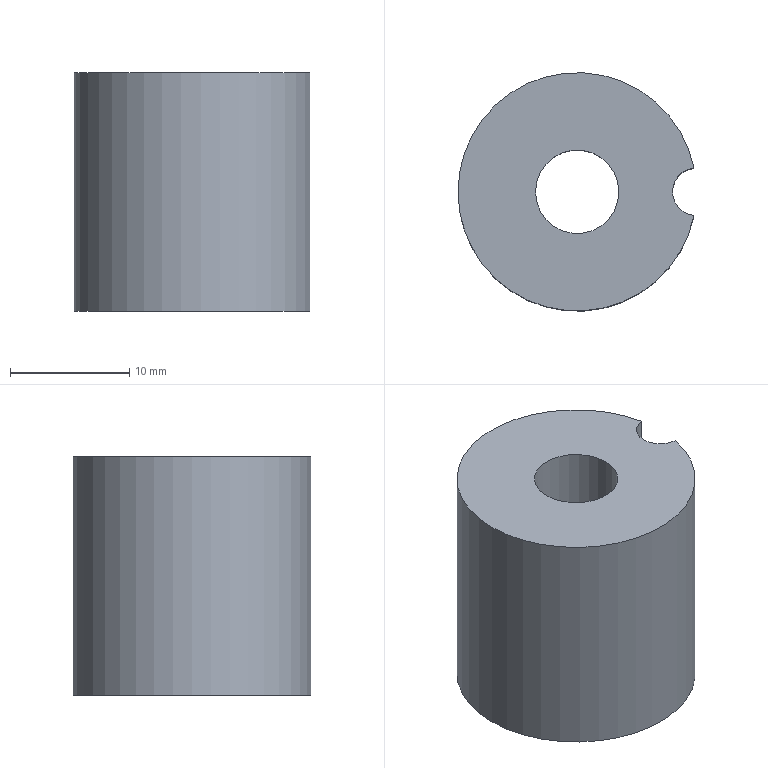Part | NX | features solid 2 | 1 solid | 7 faces | box 19.8 x 20 x 20 mm | volume 4359 mm3 | cylinder 4 | plane 3 | commonest cylinder face diameters 4 x1 7 x1 12.6 x1 20 x1
STEP:
#1=CARTESIAN_POINT('',(323.925,42.82,65.568));
#2=VERTEX_POINT('',#1);
#3=CARTESIAN_POINT('',(323.925,42.82,85.568));
#4=VERTEX_POINT('',#3);
#5=CARTESIAN_POINT('',(323.925,42.82,75.568));
#6=DIRECTION('',(0.,0.,1.));
#7=VECTOR('',#6,1000.);
#8=LINE('',#5,#7);
#9=EDGE_CURVE('',#2,#4,#8,.T.);
#10=ORIENTED_EDGE('',*,*,#9,.F.);
#11=CARTESIAN_POINT('',(323.925,38.84,65.568));
#12=VERTEX_POINT('',#11);
#13=CARTESIAN_POINT('',(314.125,40.83,65.568));
#14=DIRECTION('',(0.,0.,1.));
#15=DIRECTION('',(1.,0.,0.));
#16=AXIS2_PLACEMENT_3D('',#13,#14,#15);
#17=CIRCLE('',#16,10.);
#18=EDGE_CURVE('',#2,#12,#17,.T.);
#19=ORIENTED_EDGE('',*,*,#18,.T.);
#20=CARTESIAN_POINT('',(323.925,38.84,85.568));
#21=VERTEX_POINT('',#20);
#22=CARTESIAN_POINT('',(323.925,38.84,75.568));
#23=DIRECTION('',(0.,0.,1.));
#24=VECTOR('',#23,1000.);
#25=LINE('',#22,#24);
#26=EDGE_CURVE('',#21,#12,#25,.F.);
#27=ORIENTED_EDGE('',*,*,#26,.F.);
#28=CARTESIAN_POINT('',(314.125,40.83,85.568));
#29=DIRECTION('',(0.,0.,1.));
#30=DIRECTION('',(1.,0.,0.));
#31=AXIS2_PLACEMENT_3D('',#28,#29,#30);
#32=CIRCLE('',#31,10.);
#33=EDGE_CURVE('',#4,#21,#32,.T.);
#34=ORIENTED_EDGE('',*,*,#33,.F.);
#35=EDGE_LOOP('',(#10,#19,#27,#34));
#36=FACE_BOUND('',#35,.T.);
#37=CARTESIAN_POINT('',(314.125,40.83,65.568));
#38=DIRECTION('',(0.,0.,1.));
#39=DIRECTION('',(1.,0.,0.));
#40=AXIS2_PLACEMENT_3D('',#37,#38,#39);
#41=CYLINDRICAL_SURFACE('',#40,10.);
#42=ADVANCED_FACE('',(#36),#41,.T.);
#43=CARTESIAN_POINT('',(320.425,40.83,65.568));
#44=VERTEX_POINT('',#43);
#45=CARTESIAN_POINT('',(314.125,40.83,65.568));
#46=DIRECTION('',(0.,0.,1.));
#47=DIRECTION('',(1.,0.,0.));
#48=AXIS2_PLACEMENT_3D('',#45,#46,#47);
#49=CIRCLE('',#48,6.3);
#50=EDGE_CURVE('',#44,#44,#49,.T.);
#51=ORIENTED_EDGE('',*,*,#50,.T.);
#52=EDGE_LOOP('',(#51));
#53=FACE_BOUND('',#52,.T.);
#54=ORIENTED_EDGE('',*,*,#18,.F.);
#55=CARTESIAN_POINT('',(324.125,40.83,65.568));
#56=DIRECTION('',(0.,0.,1.));
#57=DIRECTION('',(1.,0.,0.));
#58=AXIS2_PLACEMENT_3D('',#55,#56,#57);
#59=CIRCLE('',#58,2.);
#60=EDGE_CURVE('',#2,#12,#59,.T.);
#61=ORIENTED_EDGE('',*,*,#60,.T.);
#62=EDGE_LOOP('',(#54,#61));
#63=FACE_BOUND('',#62,.T.);
#64=CARTESIAN_POINT('',(314.125,40.83,65.568));
#65=DIRECTION('',(0.,0.,1.));
#66=DIRECTION('',(1.,0.,0.));
#67=AXIS2_PLACEMENT_3D('',#64,#65,#66);
#68=PLANE('',#67);
#69=ADVANCED_FACE('',(#53,#63),#68,.F.);
#70=CARTESIAN_POINT('',(317.625,40.83,85.568));
#71=VERTEX_POINT('',#70);
#72=CARTESIAN_POINT('',(314.125,40.83,85.568));
#73=DIRECTION('',(0.,0.,1.));
#74=DIRECTION('',(1.,0.,0.));
#75=AXIS2_PLACEMENT_3D('',#72,#73,#74);
#76=CIRCLE('',#75,3.5);
#77=EDGE_CURVE('',#71,#71,#76,.T.);
#78=ORIENTED_EDGE('',*,*,#77,.F.);
#79=EDGE_LOOP('',(#78));
#80=FACE_BOUND('',#79,.T.);
#81=CARTESIAN_POINT('',(324.125,40.83,85.568));
#82=DIRECTION('',(0.,0.,1.));
#83=DIRECTION('',(1.,0.,0.));
#84=AXIS2_PLACEMENT_3D('',#81,#82,#83);
#85=CIRCLE('',#84,2.);
#86=EDGE_CURVE('',#4,#21,#85,.T.);
#87=ORIENTED_EDGE('',*,*,#86,.F.);
#88=ORIENTED_EDGE('',*,*,#33,.T.);
#89=EDGE_LOOP('',(#87,#88));
#90=FACE_BOUND('',#89,.T.);
#91=CARTESIAN_POINT('',(314.125,40.83,85.568));
#92=DIRECTION('',(0.,0.,1.));
#93=DIRECTION('',(1.,0.,0.));
#94=AXIS2_PLACEMENT_3D('',#91,#92,#93);
#95=PLANE('',#94);
#96=ADVANCED_FACE('',(#80,#90),#95,.T.);
#97=ORIENTED_EDGE('',*,*,#50,.F.);
#98=EDGE_LOOP('',(#97));
#99=FACE_BOUND('',#98,.T.);
#100=CARTESIAN_POINT('',(320.425,40.83,77.568));
#101=VERTEX_POINT('',#100);
#102=CARTESIAN_POINT('',(314.125,40.83,77.568));
#103=DIRECTION('',(0.,0.,1.));
#104=DIRECTION('',(1.,0.,0.));
#105=AXIS2_PLACEMENT_3D('',#102,#103,#104);
#106=CIRCLE('',#105,6.3);
#107=EDGE_CURVE('',#101,#101,#106,.T.);
#108=ORIENTED_EDGE('',*,*,#107,.T.);
#109=EDGE_LOOP('',(#108));
#110=FACE_BOUND('',#109,.T.);
#111=CARTESIAN_POINT('',(314.125,40.83,65.568));
#112=DIRECTION('',(0.,0.,1.));
#113=DIRECTION('',(1.,0.,0.));
#114=AXIS2_PLACEMENT_3D('',#111,#112,#113);
#115=CYLINDRICAL_SURFACE('',#114,6.3);
#116=ADVANCED_FACE('',(#99,#110),#115,.F.);
#117=CARTESIAN_POINT('',(317.625,40.83,77.568));
#118=VERTEX_POINT('',#117);
#119=CARTESIAN_POINT('',(314.125,40.83,77.568));
#120=DIRECTION('',(0.,0.,1.));
#121=DIRECTION('',(1.,0.,0.));
#122=AXIS2_PLACEMENT_3D('',#119,#120,#121);
#123=CIRCLE('',#122,3.5);
#124=EDGE_CURVE('',#118,#118,#123,.T.);
#125=ORIENTED_EDGE('',*,*,#124,.T.);
#126=EDGE_LOOP('',(#125));
#127=FACE_BOUND('',#126,.T.);
#128=ORIENTED_EDGE('',*,*,#107,.F.);
#129=EDGE_LOOP('',(#128));
#130=FACE_BOUND('',#129,.T.);
#131=CARTESIAN_POINT('',(314.125,40.83,77.568));
#132=DIRECTION('',(0.,0.,1.));
#133=DIRECTION('',(1.,0.,0.));
#134=AXIS2_PLACEMENT_3D('',#131,#132,#133);
#135=PLANE('',#134);
#136=ADVANCED_FACE('',(#127,#130),#135,.F.);
#137=ORIENTED_EDGE('',*,*,#9,.T.);
#138=ORIENTED_EDGE('',*,*,#86,.T.);
#139=ORIENTED_EDGE('',*,*,#26,.T.);
#140=ORIENTED_EDGE('',*,*,#60,.F.);
#141=EDGE_LOOP('',(#137,#138,#139,#140));
#142=FACE_BOUND('',#141,.T.);
#143=CARTESIAN_POINT('',(324.125,40.83,65.568));
#144=DIRECTION('',(0.,0.,1.));
#145=DIRECTION('',(1.,0.,0.));
#146=AXIS2_PLACEMENT_3D('',#143,#144,#145);
#147=CYLINDRICAL_SURFACE('',#146,2.);
#148=ADVANCED_FACE('',(#142),#147,.F.);
#149=ORIENTED_EDGE('',*,*,#77,.T.);
#150=EDGE_LOOP('',(#149));
#151=FACE_BOUND('',#150,.T.);
#152=ORIENTED_EDGE('',*,*,#124,.F.);
#153=EDGE_LOOP('',(#152));
#154=FACE_BOUND('',#153,.T.);
#155=CARTESIAN_POINT('',(314.125,40.83,65.568));
#156=DIRECTION('',(0.,0.,1.));
#157=DIRECTION('',(1.,0.,0.));
#158=AXIS2_PLACEMENT_3D('',#155,#156,#157);
#159=CYLINDRICAL_SURFACE('',#158,3.5);
#160=ADVANCED_FACE('',(#151,#154),#159,.F.);
#161=CLOSED_SHELL('',(#42,#69,#96,#116,#136,#148,#160));
#162=MANIFOLD_SOLID_BREP('',#161);
#163=(LENGTH_UNIT()NAMED_UNIT(*)SI_UNIT(.MILLI.,.METRE.));
#164=UNCERTAINTY_MEASURE_WITH_UNIT(LENGTH_MEASURE(0.00001),#163,'','');
#165=(NAMED_UNIT(*)PLANE_ANGLE_UNIT()SI_UNIT($,.RADIAN.));
#166=(NAMED_UNIT(*)SI_UNIT($,.STERADIAN.)SOLID_ANGLE_UNIT());
#167=(GEOMETRIC_REPRESENTATION_CONTEXT(3)GLOBAL_UNCERTAINTY_ASSIGNED_CONTEXT((#164))GLOBAL_UNIT_ASSIGNED_CONTEXT((#163,#165,#166))REPRESENTATION_CONTEXT('',''));
#168=ADVANCED_BREP_SHAPE_REPRESENTATION('',(#162),#167);